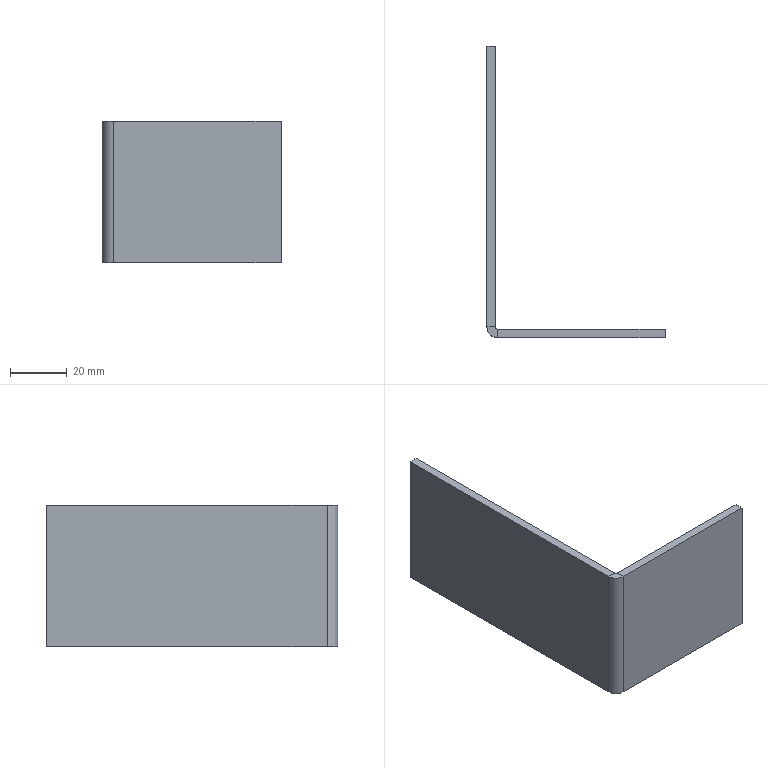Part | STEP file | MYT-A01-P30 | 1 solid | 14 faces | box 63 x 103 x 50 mm | volume 24306 mm3 | plane 12 | cylinder 2 | commonest cylinder face diameters 1.473 x1 7.473 x1
STEP:
#1=CARTESIAN_POINT('',(0.7366,0.,25.));
#2=VERTEX_POINT('',#1);
#3=CARTESIAN_POINT('',(0.7366,-3.,25.));
#4=VERTEX_POINT('',#3);
#5=CARTESIAN_POINT('',(0.7366,0.,25.));
#6=DIRECTION('',(0.,-1.,0.));
#7=VECTOR('',#6,1000.);
#8=LINE('',#5,#7);
#9=EDGE_CURVE('',#2,#4,#8,.T.);
#10=ORIENTED_EDGE('',*,*,#9,.F.);
#11=CARTESIAN_POINT('',(0.,0.7366,25.));
#12=VERTEX_POINT('',#11);
#13=CARTESIAN_POINT('',(0.7366,0.7366,25.));
#14=DIRECTION('',(0.,0.,1.));
#15=DIRECTION('',(-1.,0.,0.));
#16=AXIS2_PLACEMENT_3D('',#13,#14,#15);
#17=CIRCLE('',#16,0.7366);
#18=EDGE_CURVE('',#12,#2,#17,.T.);
#19=ORIENTED_EDGE('',*,*,#18,.F.);
#20=CARTESIAN_POINT('',(-3.,0.7366,25.));
#21=VERTEX_POINT('',#20);
#22=CARTESIAN_POINT('',(-3.,0.7366,25.));
#23=DIRECTION('',(1.,0.,0.));
#24=VECTOR('',#23,1000.);
#25=LINE('',#22,#24);
#26=EDGE_CURVE('',#21,#12,#25,.T.);
#27=ORIENTED_EDGE('',*,*,#26,.F.);
#28=CARTESIAN_POINT('',(0.7366,0.7366,25.));
#29=DIRECTION('',(0.,0.,1.));
#30=DIRECTION('',(1.,0.,0.));
#31=AXIS2_PLACEMENT_3D('',#28,#29,#30);
#32=CIRCLE('',#31,3.737);
#33=EDGE_CURVE('',#21,#4,#32,.T.);
#34=ORIENTED_EDGE('',*,*,#33,.T.);
#35=EDGE_LOOP('',(#10,#19,#27,#34));
#36=FACE_OUTER_BOUND('',#35,.T.);
#37=CARTESIAN_POINT('',(0.7366,0.,25.));
#38=DIRECTION('',(0.,0.,1.));
#39=DIRECTION('',(1.,0.,0.));
#40=AXIS2_PLACEMENT_3D('',#37,#38,#39);
#41=PLANE('',#40);
#42=ADVANCED_FACE('',(#36),#41,.T.);
#43=CARTESIAN_POINT('',(60.,0.,25.));
#44=VERTEX_POINT('',#43);
#45=CARTESIAN_POINT('',(0.,0.,25.));
#46=DIRECTION('',(1.,0.,0.));
#47=VECTOR('',#46,1000.);
#48=LINE('',#45,#47);
#49=EDGE_CURVE('',#2,#44,#48,.T.);
#50=ORIENTED_EDGE('',*,*,#49,.F.);
#51=ORIENTED_EDGE('',*,*,#9,.T.);
#52=CARTESIAN_POINT('',(60.,-3.,25.));
#53=VERTEX_POINT('',#52);
#54=CARTESIAN_POINT('',(0.,-3.,25.));
#55=DIRECTION('',(1.,0.,0.));
#56=VECTOR('',#55,1000.);
#57=LINE('',#54,#56);
#58=EDGE_CURVE('',#4,#53,#57,.T.);
#59=ORIENTED_EDGE('',*,*,#58,.T.);
#60=CARTESIAN_POINT('',(60.,0.,25.));
#61=DIRECTION('',(0.,-1.,0.));
#62=VECTOR('',#61,1000.);
#63=LINE('',#60,#62);
#64=EDGE_CURVE('',#44,#53,#63,.T.);
#65=ORIENTED_EDGE('',*,*,#64,.F.);
#66=EDGE_LOOP('',(#50,#51,#59,#65));
#67=FACE_OUTER_BOUND('',#66,.T.);
#68=CARTESIAN_POINT('',(-3.,0.7366,25.));
#69=DIRECTION('',(0.,0.,1.));
#70=DIRECTION('',(1.,0.,0.));
#71=AXIS2_PLACEMENT_3D('',#68,#69,#70);
#72=PLANE('',#71);
#73=ADVANCED_FACE('',(#67),#72,.T.);
#74=CARTESIAN_POINT('',(0.,0.7366,-25.));
#75=VERTEX_POINT('',#74);
#76=CARTESIAN_POINT('',(-3.,0.7366,-25.));
#77=VERTEX_POINT('',#76);
#78=CARTESIAN_POINT('',(0.,0.7366,-25.));
#79=DIRECTION('',(-1.,0.,0.));
#80=VECTOR('',#79,1000.);
#81=LINE('',#78,#80);
#82=EDGE_CURVE('',#75,#77,#81,.T.);
#83=ORIENTED_EDGE('',*,*,#82,.F.);
#84=CARTESIAN_POINT('',(0.7366,0.,-25.));
#85=VERTEX_POINT('',#84);
#86=CARTESIAN_POINT('',(0.7366,0.7366,-25.));
#87=DIRECTION('',(0.,0.,1.));
#88=DIRECTION('',(-1.,0.,0.));
#89=AXIS2_PLACEMENT_3D('',#86,#87,#88);
#90=CIRCLE('',#89,0.7366);
#91=EDGE_CURVE('',#75,#85,#90,.T.);
#92=ORIENTED_EDGE('',*,*,#91,.T.);
#93=CARTESIAN_POINT('',(0.7366,-3.,-25.));
#94=VERTEX_POINT('',#93);
#95=CARTESIAN_POINT('',(0.7366,-3.,-25.));
#96=DIRECTION('',(0.,1.,0.));
#97=VECTOR('',#96,1000.);
#98=LINE('',#95,#97);
#99=EDGE_CURVE('',#94,#85,#98,.T.);
#100=ORIENTED_EDGE('',*,*,#99,.F.);
#101=CARTESIAN_POINT('',(0.7366,0.7366,-25.));
#102=DIRECTION('',(0.,0.,1.));
#103=DIRECTION('',(1.,0.,0.));
#104=AXIS2_PLACEMENT_3D('',#101,#102,#103);
#105=CIRCLE('',#104,3.737);
#106=EDGE_CURVE('',#77,#94,#105,.T.);
#107=ORIENTED_EDGE('',*,*,#106,.F.);
#108=EDGE_LOOP('',(#83,#92,#100,#107));
#109=FACE_OUTER_BOUND('',#108,.T.);
#110=CARTESIAN_POINT('',(0.,0.7366,-25.));
#111=DIRECTION('',(0.,0.,-1.));
#112=DIRECTION('',(-1.,0.,0.));
#113=AXIS2_PLACEMENT_3D('',#110,#111,#112);
#114=PLANE('',#113);
#115=ADVANCED_FACE('',(#109),#114,.T.);
#116=CARTESIAN_POINT('',(0.,100.,-25.));
#117=VERTEX_POINT('',#116);
#118=CARTESIAN_POINT('',(0.,100.,-25.));
#119=DIRECTION('',(0.,-1.,0.));
#120=VECTOR('',#119,1000.);
#121=LINE('',#118,#120);
#122=EDGE_CURVE('',#117,#75,#121,.T.);
#123=ORIENTED_EDGE('',*,*,#122,.T.);
#124=ORIENTED_EDGE('',*,*,#82,.T.);
#125=CARTESIAN_POINT('',(-3.,100.,-25.));
#126=VERTEX_POINT('',#125);
#127=CARTESIAN_POINT('',(-3.,100.,-25.));
#128=DIRECTION('',(0.,-1.,0.));
#129=VECTOR('',#128,1000.);
#130=LINE('',#127,#129);
#131=EDGE_CURVE('',#126,#77,#130,.T.);
#132=ORIENTED_EDGE('',*,*,#131,.F.);
#133=CARTESIAN_POINT('',(-3.,100.,-25.));
#134=DIRECTION('',(1.,0.,0.));
#135=VECTOR('',#134,1000.);
#136=LINE('',#133,#135);
#137=EDGE_CURVE('',#126,#117,#136,.T.);
#138=ORIENTED_EDGE('',*,*,#137,.T.);
#139=EDGE_LOOP('',(#123,#124,#132,#138));
#140=FACE_OUTER_BOUND('',#139,.T.);
#141=CARTESIAN_POINT('',(0.7366,-3.,-25.));
#142=DIRECTION('',(0.,0.,-1.));
#143=DIRECTION('',(-1.,0.,0.));
#144=AXIS2_PLACEMENT_3D('',#141,#142,#143);
#145=PLANE('',#144);
#146=ADVANCED_FACE('',(#140),#145,.T.);
#147=CARTESIAN_POINT('',(60.,-3.,-25.));
#148=VERTEX_POINT('',#147);
#149=CARTESIAN_POINT('',(0.,-3.,-25.));
#150=DIRECTION('',(1.,0.,0.));
#151=VECTOR('',#150,1000.);
#152=LINE('',#149,#151);
#153=EDGE_CURVE('',#94,#148,#152,.T.);
#154=ORIENTED_EDGE('',*,*,#153,.T.);
#155=CARTESIAN_POINT('',(60.,-3.,25.));
#156=DIRECTION('',(0.,0.,-1.));
#157=VECTOR('',#156,1000.);
#158=LINE('',#155,#157);
#159=EDGE_CURVE('',#53,#148,#158,.T.);
#160=ORIENTED_EDGE('',*,*,#159,.F.);
#161=ORIENTED_EDGE('',*,*,#58,.F.);
#162=CARTESIAN_POINT('',(0.7366,-3.,25.));
#163=DIRECTION('',(0.,0.,-1.));
#164=VECTOR('',#163,1000.);
#165=LINE('',#162,#164);
#166=EDGE_CURVE('',#4,#94,#165,.T.);
#167=ORIENTED_EDGE('',*,*,#166,.T.);
#168=EDGE_LOOP('',(#154,#160,#161,#167));
#169=FACE_OUTER_BOUND('',#168,.T.);
#170=CARTESIAN_POINT('',(0.,-3.,25.));
#171=DIRECTION('',(0.,1.,0.));
#172=DIRECTION('',(0.,0.,1.));
#173=AXIS2_PLACEMENT_3D('',#170,#171,#172);
#174=PLANE('',#173);
#175=ADVANCED_FACE('',(#169),#174,.F.);
#176=CARTESIAN_POINT('',(60.,0.,-25.));
#177=VERTEX_POINT('',#176);
#178=CARTESIAN_POINT('',(60.,0.,-25.));
#179=DIRECTION('',(0.,-1.,0.));
#180=VECTOR('',#179,1000.);
#181=LINE('',#178,#180);
#182=EDGE_CURVE('',#177,#148,#181,.T.);
#183=ORIENTED_EDGE('',*,*,#182,.F.);
#184=CARTESIAN_POINT('',(60.,0.,25.));
#185=DIRECTION('',(0.,0.,-1.));
#186=VECTOR('',#185,1000.);
#187=LINE('',#184,#186);
#188=EDGE_CURVE('',#44,#177,#187,.T.);
#189=ORIENTED_EDGE('',*,*,#188,.F.);
#190=ORIENTED_EDGE('',*,*,#64,.T.);
#191=ORIENTED_EDGE('',*,*,#159,.T.);
#192=EDGE_LOOP('',(#183,#189,#190,#191));
#193=FACE_OUTER_BOUND('',#192,.T.);
#194=CARTESIAN_POINT('',(60.,0.,25.));
#195=DIRECTION('',(1.,0.,0.));
#196=DIRECTION('',(0.,0.,-1.));
#197=AXIS2_PLACEMENT_3D('',#194,#195,#196);
#198=PLANE('',#197);
#199=ADVANCED_FACE('',(#193),#198,.T.);
#200=CARTESIAN_POINT('',(0.,0.,-25.));
#201=DIRECTION('',(1.,0.,0.));
#202=VECTOR('',#201,1000.);
#203=LINE('',#200,#202);
#204=EDGE_CURVE('',#85,#177,#203,.T.);
#205=ORIENTED_EDGE('',*,*,#204,.F.);
#206=CARTESIAN_POINT('',(0.7366,0.,25.));
#207=DIRECTION('',(0.,0.,-1.));
#208=VECTOR('',#207,1000.);
#209=LINE('',#206,#208);
#210=EDGE_CURVE('',#2,#85,#209,.T.);
#211=ORIENTED_EDGE('',*,*,#210,.F.);
#212=ORIENTED_EDGE('',*,*,#49,.T.);
#213=ORIENTED_EDGE('',*,*,#188,.T.);
#214=EDGE_LOOP('',(#205,#211,#212,#213));
#215=FACE_OUTER_BOUND('',#214,.T.);
#216=CARTESIAN_POINT('',(0.,0.,25.));
#217=DIRECTION('',(0.,1.,0.));
#218=DIRECTION('',(0.,0.,1.));
#219=AXIS2_PLACEMENT_3D('',#216,#217,#218);
#220=PLANE('',#219);
#221=ADVANCED_FACE('',(#215),#220,.T.);
#222=ORIENTED_EDGE('',*,*,#91,.F.);
#223=CARTESIAN_POINT('',(0.,0.7366,25.));
#224=DIRECTION('',(0.,0.,-1.));
#225=VECTOR('',#224,1000.);
#226=LINE('',#223,#225);
#227=EDGE_CURVE('',#12,#75,#226,.T.);
#228=ORIENTED_EDGE('',*,*,#227,.F.);
#229=ORIENTED_EDGE('',*,*,#18,.T.);
#230=ORIENTED_EDGE('',*,*,#210,.T.);
#231=EDGE_LOOP('',(#222,#228,#229,#230));
#232=FACE_OUTER_BOUND('',#231,.T.);
#233=CARTESIAN_POINT('',(0.7366,0.7366,25.));
#234=DIRECTION('',(0.,0.,-1.));
#235=DIRECTION('',(-1.,0.,0.));
#236=AXIS2_PLACEMENT_3D('',#233,#234,#235);
#237=CYLINDRICAL_SURFACE('',#236,0.7366);
#238=ADVANCED_FACE('',(#232),#237,.F.);
#239=ORIENTED_EDGE('',*,*,#122,.F.);
#240=CARTESIAN_POINT('',(0.,100.,25.));
#241=VERTEX_POINT('',#240);
#242=CARTESIAN_POINT('',(0.,100.,25.));
#243=DIRECTION('',(0.,0.,-1.));
#244=VECTOR('',#243,1000.);
#245=LINE('',#242,#244);
#246=EDGE_CURVE('',#241,#117,#245,.T.);
#247=ORIENTED_EDGE('',*,*,#246,.F.);
#248=CARTESIAN_POINT('',(0.,100.,25.));
#249=DIRECTION('',(0.,-1.,0.));
#250=VECTOR('',#249,1000.);
#251=LINE('',#248,#250);
#252=EDGE_CURVE('',#241,#12,#251,.T.);
#253=ORIENTED_EDGE('',*,*,#252,.T.);
#254=ORIENTED_EDGE('',*,*,#227,.T.);
#255=EDGE_LOOP('',(#239,#247,#253,#254));
#256=FACE_OUTER_BOUND('',#255,.T.);
#257=CARTESIAN_POINT('',(0.,100.,25.));
#258=DIRECTION('',(1.,0.,0.));
#259=DIRECTION('',(0.,0.,-1.));
#260=AXIS2_PLACEMENT_3D('',#257,#258,#259);
#261=PLANE('',#260);
#262=ADVANCED_FACE('',(#256),#261,.T.);
#263=ORIENTED_EDGE('',*,*,#137,.F.);
#264=CARTESIAN_POINT('',(-3.,100.,25.));
#265=VERTEX_POINT('',#264);
#266=CARTESIAN_POINT('',(-3.,100.,25.));
#267=DIRECTION('',(0.,0.,-1.));
#268=VECTOR('',#267,1000.);
#269=LINE('',#266,#268);
#270=EDGE_CURVE('',#265,#126,#269,.T.);
#271=ORIENTED_EDGE('',*,*,#270,.F.);
#272=CARTESIAN_POINT('',(-3.,100.,25.));
#273=DIRECTION('',(1.,0.,0.));
#274=VECTOR('',#273,1000.);
#275=LINE('',#272,#274);
#276=EDGE_CURVE('',#265,#241,#275,.T.);
#277=ORIENTED_EDGE('',*,*,#276,.T.);
#278=ORIENTED_EDGE('',*,*,#246,.T.);
#279=EDGE_LOOP('',(#263,#271,#277,#278));
#280=FACE_OUTER_BOUND('',#279,.T.);
#281=CARTESIAN_POINT('',(-3.,100.,25.));
#282=DIRECTION('',(0.,1.,0.));
#283=DIRECTION('',(0.,0.,1.));
#284=AXIS2_PLACEMENT_3D('',#281,#282,#283);
#285=PLANE('',#284);
#286=ADVANCED_FACE('',(#280),#285,.T.);
#287=ORIENTED_EDGE('',*,*,#131,.T.);
#288=CARTESIAN_POINT('',(-3.,0.7366,25.));
#289=DIRECTION('',(0.,0.,-1.));
#290=VECTOR('',#289,1000.);
#291=LINE('',#288,#290);
#292=EDGE_CURVE('',#21,#77,#291,.T.);
#293=ORIENTED_EDGE('',*,*,#292,.F.);
#294=CARTESIAN_POINT('',(-3.,100.,25.));
#295=DIRECTION('',(0.,-1.,0.));
#296=VECTOR('',#295,1000.);
#297=LINE('',#294,#296);
#298=EDGE_CURVE('',#265,#21,#297,.T.);
#299=ORIENTED_EDGE('',*,*,#298,.F.);
#300=ORIENTED_EDGE('',*,*,#270,.T.);
#301=EDGE_LOOP('',(#287,#293,#299,#300));
#302=FACE_OUTER_BOUND('',#301,.T.);
#303=CARTESIAN_POINT('',(-3.,100.,25.));
#304=DIRECTION('',(1.,0.,0.));
#305=DIRECTION('',(0.,0.,-1.));
#306=AXIS2_PLACEMENT_3D('',#303,#304,#305);
#307=PLANE('',#306);
#308=ADVANCED_FACE('',(#302),#307,.F.);
#309=ORIENTED_EDGE('',*,*,#106,.T.);
#310=ORIENTED_EDGE('',*,*,#166,.F.);
#311=ORIENTED_EDGE('',*,*,#33,.F.);
#312=ORIENTED_EDGE('',*,*,#292,.T.);
#313=EDGE_LOOP('',(#309,#310,#311,#312));
#314=FACE_OUTER_BOUND('',#313,.T.);
#315=CARTESIAN_POINT('',(0.7366,0.7366,25.));
#316=DIRECTION('',(0.,0.,-1.));
#317=DIRECTION('',(-1.,0.,0.));
#318=AXIS2_PLACEMENT_3D('',#315,#316,#317);
#319=CYLINDRICAL_SURFACE('',#318,3.737);
#320=ADVANCED_FACE('',(#314),#319,.T.);
#321=ORIENTED_EDGE('',*,*,#298,.T.);
#322=ORIENTED_EDGE('',*,*,#26,.T.);
#323=ORIENTED_EDGE('',*,*,#252,.F.);
#324=ORIENTED_EDGE('',*,*,#276,.F.);
#325=EDGE_LOOP('',(#321,#322,#323,#324));
#326=FACE_OUTER_BOUND('',#325,.T.);
#327=CARTESIAN_POINT('',(0.7366,0.7366,25.));
#328=DIRECTION('',(0.,0.,-1.));
#329=DIRECTION('',(-1.,0.,0.));
#330=AXIS2_PLACEMENT_3D('',#327,#328,#329);
#331=PLANE('',#330);
#332=ADVANCED_FACE('',(#326),#331,.F.);
#333=ORIENTED_EDGE('',*,*,#153,.F.);
#334=ORIENTED_EDGE('',*,*,#99,.T.);
#335=ORIENTED_EDGE('',*,*,#204,.T.);
#336=ORIENTED_EDGE('',*,*,#182,.T.);
#337=EDGE_LOOP('',(#333,#334,#335,#336));
#338=FACE_OUTER_BOUND('',#337,.T.);
#339=CARTESIAN_POINT('',(0.7366,0.7366,-25.));
#340=DIRECTION('',(0.,0.,-1.));
#341=DIRECTION('',(-1.,0.,0.));
#342=AXIS2_PLACEMENT_3D('',#339,#340,#341);
#343=PLANE('',#342);
#344=ADVANCED_FACE('',(#338),#343,.T.);
#345=CLOSED_SHELL('',(#42,#73,#115,#146,#175,#199,#221,#238,#262,#286,#308,#320,#332,#344));
#346=MANIFOLD_SOLID_BREP('',#345);
#347=CARTESIAN_POINT('',(0.,0.,0.));
#348=DIRECTION('',(0.,0.,1.));
#349=DIRECTION('',(1.,0.,0.));
#350=AXIS2_PLACEMENT_3D('',#347,#348,#349);
#351=(LENGTH_UNIT()NAMED_UNIT(*)SI_UNIT(.MILLI.,.METRE.));
#352=UNCERTAINTY_MEASURE_WITH_UNIT(LENGTH_MEASURE(0.00001),#351,'','');
#353=(NAMED_UNIT(*)PLANE_ANGLE_UNIT()SI_UNIT($,.RADIAN.));
#354=(NAMED_UNIT(*)SI_UNIT($,.STERADIAN.)SOLID_ANGLE_UNIT());
#355=(GEOMETRIC_REPRESENTATION_CONTEXT(3)GLOBAL_UNCERTAINTY_ASSIGNED_CONTEXT((#352))GLOBAL_UNIT_ASSIGNED_CONTEXT((#351,#353,#354))REPRESENTATION_CONTEXT('',''));
#356=ADVANCED_BREP_SHAPE_REPRESENTATION('',(#346,#350),#355);